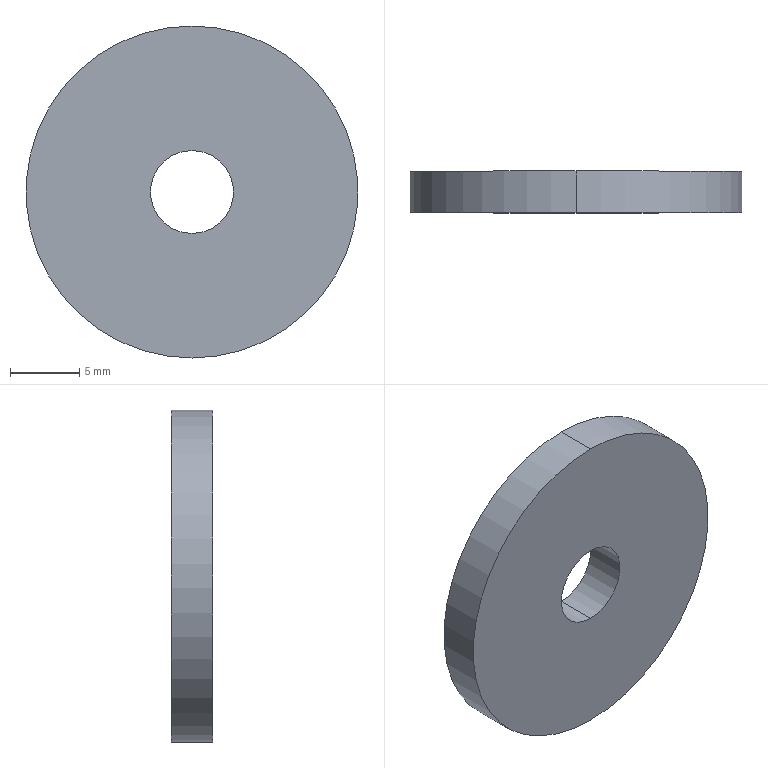Part | STEP file | 1 solid | 6 faces | box 24 x 3 x 24 mm | volume 1272 mm3 | cylinder 4 | plane 2 | commonest cylinder face diameters 6 x2 24 x2
STEP:
#1=CARTESIAN_POINT('',(0.,0.,0.));
#2=DIRECTION('',(0.,0.,1.));
#3=DIRECTION('',(1.,0.,0.));
#4=AXIS2_PLACEMENT_3D('',#1,#2,#3);
#5=CARTESIAN_POINT('',(0.,0.,12.));
#6=VERTEX_POINT('',#5);
#7=CARTESIAN_POINT('',(0.,0.,-12.));
#8=VERTEX_POINT('',#7);
#9=CARTESIAN_POINT('',(0.,0.,0.));
#10=DIRECTION('',(0.,1.,0.));
#11=DIRECTION('',(0.,0.,1.));
#12=AXIS2_PLACEMENT_3D('',#9,#10,#11);
#13=CIRCLE('',#12,12.);
#14=CARTESIAN_POINT('',(0.,0.,0.));
#15=DIRECTION('',(0.,1.,0.));
#16=DIRECTION('',(0.,0.,1.));
#17=AXIS2_PLACEMENT_3D('',#14,#15,#16);
#18=CYLINDRICAL_SURFACE('',#17,12.);
#19=CARTESIAN_POINT('',(0.,0.));
#20=DIRECTION('',(1.,0.));
#21=VECTOR('',#20,1.);
#22=LINE('',#19,#21);
#23=(GEOMETRIC_REPRESENTATION_CONTEXT(2)PARAMETRIC_REPRESENTATION_CONTEXT()REPRESENTATION_CONTEXT('',''));
#24=DEFINITIONAL_REPRESENTATION('',(#22),#23);
#25=PCURVE('',#18,#24);
#26=CARTESIAN_POINT('',(0.,0.,0.));
#27=DIRECTION('',(0.,1.,0.));
#28=DIRECTION('',(0.,0.,1.));
#29=AXIS2_PLACEMENT_3D('',#26,#27,#28);
#30=PLANE('',#29);
#31=CARTESIAN_POINT('',(0.,0.));
#32=DIRECTION('',(1.,0.));
#33=AXIS2_PLACEMENT_2D('',#31,#32);
#34=CIRCLE('',#33,12.);
#35=(GEOMETRIC_REPRESENTATION_CONTEXT(2)PARAMETRIC_REPRESENTATION_CONTEXT()REPRESENTATION_CONTEXT('',''));
#36=DEFINITIONAL_REPRESENTATION('',(#34),#35);
#37=PCURVE('',#30,#36);
#38=SURFACE_CURVE('',#13,(#25,#37),.PCURVE_S1.);
#39=EDGE_CURVE('',#6,#8,#38,.T.);
#40=ORIENTED_EDGE('',*,*,#39,.T.);
#41=CARTESIAN_POINT('',(0.,3.,-12.));
#42=VERTEX_POINT('',#41);
#43=CARTESIAN_POINT('',(0.,0.,-12.));
#44=DIRECTION('',(0.,1.,0.));
#45=VECTOR('',#44,1.);
#46=LINE('',#43,#45);
#47=CARTESIAN_POINT('',(3.142,0.));
#48=DIRECTION('',(0.,1.));
#49=VECTOR('',#48,1.);
#50=LINE('',#47,#49);
#51=(GEOMETRIC_REPRESENTATION_CONTEXT(2)PARAMETRIC_REPRESENTATION_CONTEXT()REPRESENTATION_CONTEXT('',''));
#52=DEFINITIONAL_REPRESENTATION('',(#50),#51);
#53=PCURVE('',#18,#52);
#54=CARTESIAN_POINT('',(0.,0.,0.));
#55=DIRECTION('',(0.,1.,0.));
#56=DIRECTION('',(0.,0.,1.));
#57=AXIS2_PLACEMENT_3D('',#54,#55,#56);
#58=CYLINDRICAL_SURFACE('',#57,12.);
#59=CARTESIAN_POINT('',(3.142,0.));
#60=DIRECTION('',(0.,1.));
#61=VECTOR('',#60,1.);
#62=LINE('',#59,#61);
#63=(GEOMETRIC_REPRESENTATION_CONTEXT(2)PARAMETRIC_REPRESENTATION_CONTEXT()REPRESENTATION_CONTEXT('',''));
#64=DEFINITIONAL_REPRESENTATION('',(#62),#63);
#65=PCURVE('',#58,#64);
#66=SURFACE_CURVE('',#46,(#53,#65),.PCURVE_S1.);
#67=EDGE_CURVE('',#8,#42,#66,.T.);
#68=ORIENTED_EDGE('',*,*,#67,.T.);
#69=CARTESIAN_POINT('',(0.,3.,12.));
#70=VERTEX_POINT('',#69);
#71=CARTESIAN_POINT('',(0.,3.,0.));
#72=DIRECTION('',(0.,1.,0.));
#73=DIRECTION('',(0.,0.,1.));
#74=AXIS2_PLACEMENT_3D('',#71,#72,#73);
#75=CIRCLE('',#74,12.);
#76=CARTESIAN_POINT('',(0.,3.));
#77=DIRECTION('',(1.,0.));
#78=VECTOR('',#77,1.);
#79=LINE('',#76,#78);
#80=(GEOMETRIC_REPRESENTATION_CONTEXT(2)PARAMETRIC_REPRESENTATION_CONTEXT()REPRESENTATION_CONTEXT('',''));
#81=DEFINITIONAL_REPRESENTATION('',(#79),#80);
#82=PCURVE('',#18,#81);
#83=CARTESIAN_POINT('',(0.,3.,0.));
#84=DIRECTION('',(0.,1.,0.));
#85=DIRECTION('',(0.,0.,1.));
#86=AXIS2_PLACEMENT_3D('',#83,#84,#85);
#87=PLANE('',#86);
#88=CARTESIAN_POINT('',(0.,0.));
#89=DIRECTION('',(1.,0.));
#90=AXIS2_PLACEMENT_2D('',#88,#89);
#91=CIRCLE('',#90,12.);
#92=(GEOMETRIC_REPRESENTATION_CONTEXT(2)PARAMETRIC_REPRESENTATION_CONTEXT()REPRESENTATION_CONTEXT('',''));
#93=DEFINITIONAL_REPRESENTATION('',(#91),#92);
#94=PCURVE('',#87,#93);
#95=SURFACE_CURVE('',#75,(#82,#94),.PCURVE_S1.);
#96=EDGE_CURVE('',#70,#42,#95,.T.);
#97=ORIENTED_EDGE('',*,*,#96,.F.);
#98=CARTESIAN_POINT('',(0.,0.,12.));
#99=DIRECTION('',(0.,1.,0.));
#100=VECTOR('',#99,1.);
#101=LINE('',#98,#100);
#102=CARTESIAN_POINT('',(0.,0.));
#103=DIRECTION('',(0.,1.));
#104=VECTOR('',#103,1.);
#105=LINE('',#102,#104);
#106=(GEOMETRIC_REPRESENTATION_CONTEXT(2)PARAMETRIC_REPRESENTATION_CONTEXT()REPRESENTATION_CONTEXT('',''));
#107=DEFINITIONAL_REPRESENTATION('',(#105),#106);
#108=PCURVE('',#18,#107);
#109=CARTESIAN_POINT('',(6.283,0.));
#110=DIRECTION('',(0.,1.));
#111=VECTOR('',#110,1.);
#112=LINE('',#109,#111);
#113=(GEOMETRIC_REPRESENTATION_CONTEXT(2)PARAMETRIC_REPRESENTATION_CONTEXT()REPRESENTATION_CONTEXT('',''));
#114=DEFINITIONAL_REPRESENTATION('',(#112),#113);
#115=PCURVE('',#58,#114);
#116=SURFACE_CURVE('',#101,(#108,#115),.PCURVE_S1.);
#117=EDGE_CURVE('',#6,#70,#116,.T.);
#118=ORIENTED_EDGE('',*,*,#117,.F.);
#119=EDGE_LOOP('',(#40,#68,#97,#118));
#120=FACE_BOUND('',#119,.T.);
#121=ADVANCED_FACE('',(#120),#18,.T.);
#122=CARTESIAN_POINT('',(0.,0.,3.));
#123=VERTEX_POINT('',#122);
#124=CARTESIAN_POINT('',(0.,3.,3.));
#125=VERTEX_POINT('',#124);
#126=CARTESIAN_POINT('',(0.,0.,3.));
#127=DIRECTION('',(0.,1.,0.));
#128=VECTOR('',#127,1.);
#129=LINE('',#126,#128);
#130=CARTESIAN_POINT('',(0.,0.,0.));
#131=DIRECTION('',(0.,1.,0.));
#132=DIRECTION('',(0.,0.,1.));
#133=AXIS2_PLACEMENT_3D('',#130,#131,#132);
#134=CYLINDRICAL_SURFACE('',#133,3.);
#135=CARTESIAN_POINT('',(6.283,0.));
#136=DIRECTION('',(0.,1.));
#137=VECTOR('',#136,1.);
#138=LINE('',#135,#137);
#139=(GEOMETRIC_REPRESENTATION_CONTEXT(2)PARAMETRIC_REPRESENTATION_CONTEXT()REPRESENTATION_CONTEXT('',''));
#140=DEFINITIONAL_REPRESENTATION('',(#138),#139);
#141=PCURVE('',#134,#140);
#142=CARTESIAN_POINT('',(0.,0.,0.));
#143=DIRECTION('',(0.,1.,0.));
#144=DIRECTION('',(0.,0.,1.));
#145=AXIS2_PLACEMENT_3D('',#142,#143,#144);
#146=CYLINDRICAL_SURFACE('',#145,3.);
#147=CARTESIAN_POINT('',(0.,0.));
#148=DIRECTION('',(0.,1.));
#149=VECTOR('',#148,1.);
#150=LINE('',#147,#149);
#151=(GEOMETRIC_REPRESENTATION_CONTEXT(2)PARAMETRIC_REPRESENTATION_CONTEXT()REPRESENTATION_CONTEXT('',''));
#152=DEFINITIONAL_REPRESENTATION('',(#150),#151);
#153=PCURVE('',#146,#152);
#154=SURFACE_CURVE('',#129,(#141,#153),.PCURVE_S1.);
#155=EDGE_CURVE('',#123,#125,#154,.T.);
#156=ORIENTED_EDGE('',*,*,#155,.T.);
#157=CARTESIAN_POINT('',(0.,3.,-3.));
#158=VERTEX_POINT('',#157);
#159=CARTESIAN_POINT('',(0.,3.,0.));
#160=DIRECTION('',(0.,-1.,0.));
#161=DIRECTION('',(0.,0.,1.));
#162=AXIS2_PLACEMENT_3D('',#159,#160,#161);
#163=CIRCLE('',#162,3.);
#164=CARTESIAN_POINT('',(6.283,3.));
#165=DIRECTION('',(-1.,0.));
#166=VECTOR('',#165,1.);
#167=LINE('',#164,#166);
#168=(GEOMETRIC_REPRESENTATION_CONTEXT(2)PARAMETRIC_REPRESENTATION_CONTEXT()REPRESENTATION_CONTEXT('',''));
#169=DEFINITIONAL_REPRESENTATION('',(#167),#168);
#170=PCURVE('',#134,#169);
#171=CARTESIAN_POINT('',(3.,0.));
#172=CARTESIAN_POINT('',(3.,-5.196));
#173=CARTESIAN_POINT('',(-1.5,-2.598));
#174=CARTESIAN_POINT('',(-6.,0.));
#175=CARTESIAN_POINT('',(-1.5,2.598));
#176=CARTESIAN_POINT('',(3.,5.196));
#177=CARTESIAN_POINT('',(3.,0.));
#178=(BOUNDED_CURVE()B_SPLINE_CURVE(2,(#171,#172,#173,#174,#175,#176,#177),.UNSPECIFIED.,.T.,.F.)B_SPLINE_CURVE_WITH_KNOTS((1,2,2,2,2,1),(-2.094,0.,2.094,4.189,6.283,8.378),.UNSPECIFIED.)CURVE()GEOMETRIC_REPRESENTATION_ITEM()RATIONAL_B_SPLINE_CURVE((1.,0.5,1.,0.5,1.,0.5,1.))REPRESENTATION_ITEM(''));
#179=(GEOMETRIC_REPRESENTATION_CONTEXT(2)PARAMETRIC_REPRESENTATION_CONTEXT()REPRESENTATION_CONTEXT('',''));
#180=DEFINITIONAL_REPRESENTATION('',(#178),#179);
#181=PCURVE('',#87,#180);
#182=SURFACE_CURVE('',#163,(#170,#181),.PCURVE_S1.);
#183=EDGE_CURVE('',#125,#158,#182,.T.);
#184=ORIENTED_EDGE('',*,*,#183,.T.);
#185=CARTESIAN_POINT('',(0.,0.,-3.));
#186=VERTEX_POINT('',#185);
#187=CARTESIAN_POINT('',(0.,0.,-3.));
#188=DIRECTION('',(0.,1.,0.));
#189=VECTOR('',#188,1.);
#190=LINE('',#187,#189);
#191=CARTESIAN_POINT('',(3.142,0.));
#192=DIRECTION('',(0.,1.));
#193=VECTOR('',#192,1.);
#194=LINE('',#191,#193);
#195=(GEOMETRIC_REPRESENTATION_CONTEXT(2)PARAMETRIC_REPRESENTATION_CONTEXT()REPRESENTATION_CONTEXT('',''));
#196=DEFINITIONAL_REPRESENTATION('',(#194),#195);
#197=PCURVE('',#134,#196);
#198=CARTESIAN_POINT('',(3.142,0.));
#199=DIRECTION('',(0.,1.));
#200=VECTOR('',#199,1.);
#201=LINE('',#198,#200);
#202=(GEOMETRIC_REPRESENTATION_CONTEXT(2)PARAMETRIC_REPRESENTATION_CONTEXT()REPRESENTATION_CONTEXT('',''));
#203=DEFINITIONAL_REPRESENTATION('',(#201),#202);
#204=PCURVE('',#146,#203);
#205=SURFACE_CURVE('',#190,(#197,#204),.PCURVE_S1.);
#206=EDGE_CURVE('',#186,#158,#205,.T.);
#207=ORIENTED_EDGE('',*,*,#206,.F.);
#208=CARTESIAN_POINT('',(0.,0.,0.));
#209=DIRECTION('',(0.,1.,0.));
#210=DIRECTION('',(0.,0.,1.));
#211=AXIS2_PLACEMENT_3D('',#208,#209,#210);
#212=CIRCLE('',#211,3.);
#213=CARTESIAN_POINT('',(0.,0.));
#214=DIRECTION('',(1.,0.));
#215=VECTOR('',#214,1.);
#216=LINE('',#213,#215);
#217=(GEOMETRIC_REPRESENTATION_CONTEXT(2)PARAMETRIC_REPRESENTATION_CONTEXT()REPRESENTATION_CONTEXT('',''));
#218=DEFINITIONAL_REPRESENTATION('',(#216),#217);
#219=PCURVE('',#134,#218);
#220=CARTESIAN_POINT('',(0.,0.));
#221=DIRECTION('',(1.,0.));
#222=AXIS2_PLACEMENT_2D('',#220,#221);
#223=CIRCLE('',#222,3.);
#224=(GEOMETRIC_REPRESENTATION_CONTEXT(2)PARAMETRIC_REPRESENTATION_CONTEXT()REPRESENTATION_CONTEXT('',''));
#225=DEFINITIONAL_REPRESENTATION('',(#223),#224);
#226=PCURVE('',#30,#225);
#227=SURFACE_CURVE('',#212,(#219,#226),.PCURVE_S1.);
#228=EDGE_CURVE('',#186,#123,#227,.T.);
#229=ORIENTED_EDGE('',*,*,#228,.T.);
#230=EDGE_LOOP('',(#156,#184,#207,#229));
#231=FACE_BOUND('',#230,.F.);
#232=ADVANCED_FACE('',(#231),#134,.F.);
#233=ORIENTED_EDGE('',*,*,#96,.T.);
#234=CARTESIAN_POINT('',(0.,3.,0.));
#235=DIRECTION('',(0.,1.,0.));
#236=DIRECTION('',(0.,0.,1.));
#237=AXIS2_PLACEMENT_3D('',#234,#235,#236);
#238=CIRCLE('',#237,12.);
#239=CARTESIAN_POINT('',(0.,0.));
#240=DIRECTION('',(1.,0.));
#241=AXIS2_PLACEMENT_2D('',#239,#240);
#242=CIRCLE('',#241,12.);
#243=(GEOMETRIC_REPRESENTATION_CONTEXT(2)PARAMETRIC_REPRESENTATION_CONTEXT()REPRESENTATION_CONTEXT('',''));
#244=DEFINITIONAL_REPRESENTATION('',(#242),#243);
#245=PCURVE('',#87,#244);
#246=CARTESIAN_POINT('',(0.,3.));
#247=DIRECTION('',(1.,0.));
#248=VECTOR('',#247,1.);
#249=LINE('',#246,#248);
#250=(GEOMETRIC_REPRESENTATION_CONTEXT(2)PARAMETRIC_REPRESENTATION_CONTEXT()REPRESENTATION_CONTEXT('',''));
#251=DEFINITIONAL_REPRESENTATION('',(#249),#250);
#252=PCURVE('',#58,#251);
#253=SURFACE_CURVE('',#238,(#245,#252),.PCURVE_S1.);
#254=EDGE_CURVE('',#42,#70,#253,.T.);
#255=ORIENTED_EDGE('',*,*,#254,.T.);
#256=EDGE_LOOP('',(#233,#255));
#257=FACE_BOUND('',#256,.T.);
#258=ORIENTED_EDGE('',*,*,#183,.T.);
#259=CARTESIAN_POINT('',(0.,3.,0.));
#260=DIRECTION('',(0.,-1.,0.));
#261=DIRECTION('',(0.,0.,1.));
#262=AXIS2_PLACEMENT_3D('',#259,#260,#261);
#263=CIRCLE('',#262,3.);
#264=CARTESIAN_POINT('',(3.,0.));
#265=CARTESIAN_POINT('',(3.,-5.196));
#266=CARTESIAN_POINT('',(-1.5,-2.598));
#267=CARTESIAN_POINT('',(-6.,0.));
#268=CARTESIAN_POINT('',(-1.5,2.598));
#269=CARTESIAN_POINT('',(3.,5.196));
#270=CARTESIAN_POINT('',(3.,0.));
#271=(BOUNDED_CURVE()B_SPLINE_CURVE(2,(#264,#265,#266,#267,#268,#269,#270),.UNSPECIFIED.,.T.,.F.)B_SPLINE_CURVE_WITH_KNOTS((1,2,2,2,2,1),(-2.094,0.,2.094,4.189,6.283,8.378),.UNSPECIFIED.)CURVE()GEOMETRIC_REPRESENTATION_ITEM()RATIONAL_B_SPLINE_CURVE((1.,0.5,1.,0.5,1.,0.5,1.))REPRESENTATION_ITEM(''));
#272=(GEOMETRIC_REPRESENTATION_CONTEXT(2)PARAMETRIC_REPRESENTATION_CONTEXT()REPRESENTATION_CONTEXT('',''));
#273=DEFINITIONAL_REPRESENTATION('',(#271),#272);
#274=PCURVE('',#87,#273);
#275=CARTESIAN_POINT('',(6.283,3.));
#276=DIRECTION('',(-1.,0.));
#277=VECTOR('',#276,1.);
#278=LINE('',#275,#277);
#279=(GEOMETRIC_REPRESENTATION_CONTEXT(2)PARAMETRIC_REPRESENTATION_CONTEXT()REPRESENTATION_CONTEXT('',''));
#280=DEFINITIONAL_REPRESENTATION('',(#278),#279);
#281=PCURVE('',#146,#280);
#282=SURFACE_CURVE('',#263,(#274,#281),.PCURVE_S1.);
#283=EDGE_CURVE('',#158,#125,#282,.T.);
#284=ORIENTED_EDGE('',*,*,#283,.T.);
#285=EDGE_LOOP('',(#258,#284));
#286=FACE_BOUND('',#285,.T.);
#287=ADVANCED_FACE('',(#257,#286),#87,.T.);
#288=ORIENTED_EDGE('',*,*,#67,.F.);
#289=CARTESIAN_POINT('',(0.,0.,0.));
#290=DIRECTION('',(0.,1.,0.));
#291=DIRECTION('',(0.,0.,1.));
#292=AXIS2_PLACEMENT_3D('',#289,#290,#291);
#293=CIRCLE('',#292,12.);
#294=CARTESIAN_POINT('',(0.,0.));
#295=DIRECTION('',(1.,0.));
#296=VECTOR('',#295,1.);
#297=LINE('',#294,#296);
#298=(GEOMETRIC_REPRESENTATION_CONTEXT(2)PARAMETRIC_REPRESENTATION_CONTEXT()REPRESENTATION_CONTEXT('',''));
#299=DEFINITIONAL_REPRESENTATION('',(#297),#298);
#300=PCURVE('',#58,#299);
#301=CARTESIAN_POINT('',(0.,0.));
#302=DIRECTION('',(1.,0.));
#303=AXIS2_PLACEMENT_2D('',#301,#302);
#304=CIRCLE('',#303,12.);
#305=(GEOMETRIC_REPRESENTATION_CONTEXT(2)PARAMETRIC_REPRESENTATION_CONTEXT()REPRESENTATION_CONTEXT('',''));
#306=DEFINITIONAL_REPRESENTATION('',(#304),#305);
#307=PCURVE('',#30,#306);
#308=SURFACE_CURVE('',#293,(#300,#307),.PCURVE_S1.);
#309=EDGE_CURVE('',#8,#6,#308,.T.);
#310=ORIENTED_EDGE('',*,*,#309,.T.);
#311=ORIENTED_EDGE('',*,*,#117,.T.);
#312=ORIENTED_EDGE('',*,*,#254,.F.);
#313=EDGE_LOOP('',(#288,#310,#311,#312));
#314=FACE_BOUND('',#313,.T.);
#315=ADVANCED_FACE('',(#314),#58,.T.);
#316=ORIENTED_EDGE('',*,*,#283,.T.);
#317=ORIENTED_EDGE('',*,*,#155,.F.);
#318=CARTESIAN_POINT('',(0.,0.,0.));
#319=DIRECTION('',(0.,1.,0.));
#320=DIRECTION('',(0.,0.,1.));
#321=AXIS2_PLACEMENT_3D('',#318,#319,#320);
#322=CIRCLE('',#321,3.);
#323=CARTESIAN_POINT('',(0.,0.));
#324=DIRECTION('',(1.,0.));
#325=VECTOR('',#324,1.);
#326=LINE('',#323,#325);
#327=(GEOMETRIC_REPRESENTATION_CONTEXT(2)PARAMETRIC_REPRESENTATION_CONTEXT()REPRESENTATION_CONTEXT('',''));
#328=DEFINITIONAL_REPRESENTATION('',(#326),#327);
#329=PCURVE('',#146,#328);
#330=CARTESIAN_POINT('',(0.,0.));
#331=DIRECTION('',(1.,0.));
#332=AXIS2_PLACEMENT_2D('',#330,#331);
#333=CIRCLE('',#332,3.);
#334=(GEOMETRIC_REPRESENTATION_CONTEXT(2)PARAMETRIC_REPRESENTATION_CONTEXT()REPRESENTATION_CONTEXT('',''));
#335=DEFINITIONAL_REPRESENTATION('',(#333),#334);
#336=PCURVE('',#30,#335);
#337=SURFACE_CURVE('',#322,(#329,#336),.PCURVE_S1.);
#338=EDGE_CURVE('',#123,#186,#337,.T.);
#339=ORIENTED_EDGE('',*,*,#338,.T.);
#340=ORIENTED_EDGE('',*,*,#206,.T.);
#341=EDGE_LOOP('',(#316,#317,#339,#340));
#342=FACE_BOUND('',#341,.F.);
#343=ADVANCED_FACE('',(#342),#146,.F.);
#344=ORIENTED_EDGE('',*,*,#39,.F.);
#345=ORIENTED_EDGE('',*,*,#309,.F.);
#346=EDGE_LOOP('',(#344,#345));
#347=FACE_BOUND('',#346,.T.);
#348=ORIENTED_EDGE('',*,*,#338,.T.);
#349=ORIENTED_EDGE('',*,*,#228,.T.);
#350=EDGE_LOOP('',(#348,#349));
#351=FACE_BOUND('',#350,.T.);
#352=ADVANCED_FACE('',(#347,#351),#30,.F.);
#353=CLOSED_SHELL('',(#121,#232,#287,#315,#343,#352));
#354=MANIFOLD_SOLID_BREP('',#353);
#355=(LENGTH_UNIT()NAMED_UNIT(*)SI_UNIT(.MILLI.,.METRE.));
#356=UNCERTAINTY_MEASURE_WITH_UNIT(LENGTH_MEASURE(0.0000001),#355,'','');
#357=(NAMED_UNIT(*)PLANE_ANGLE_UNIT()SI_UNIT($,.RADIAN.));
#358=(NAMED_UNIT(*)SI_UNIT($,.STERADIAN.)SOLID_ANGLE_UNIT());
#359=(GEOMETRIC_REPRESENTATION_CONTEXT(3)GLOBAL_UNCERTAINTY_ASSIGNED_CONTEXT((#356))GLOBAL_UNIT_ASSIGNED_CONTEXT((#355,#357,#358))REPRESENTATION_CONTEXT('',''));
#360=ADVANCED_BREP_SHAPE_REPRESENTATION('',(#4,#354),#359);